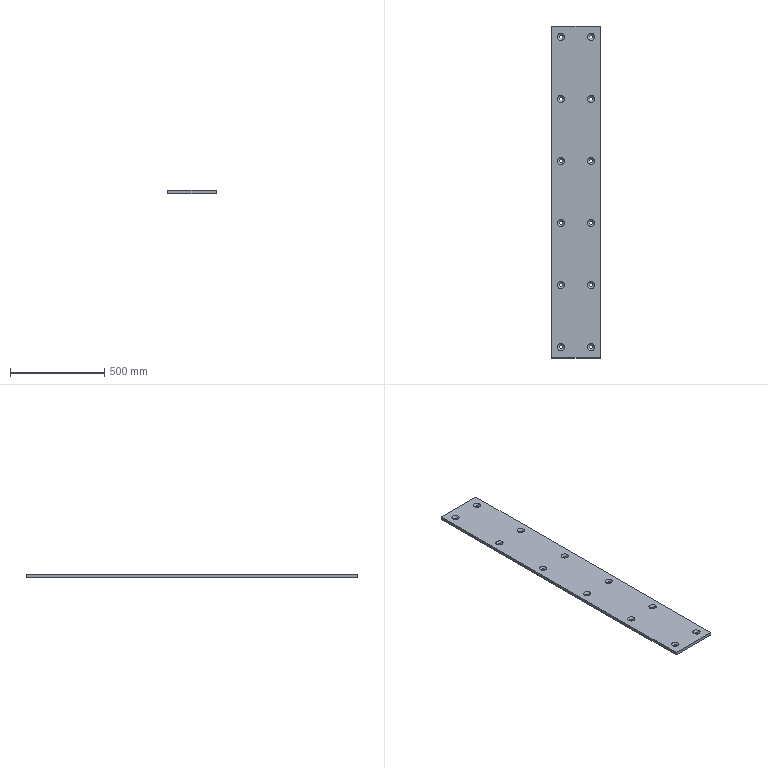Part | STEP file | Liner plate_Default<As machined> | 1 solid | 54 faces | box 260 x 1764 x 16 mm | volume 7243869 mm3 | cone 24 | cylinder 24 | plane 6 | commonest cylinder face diameters 17.5 x24